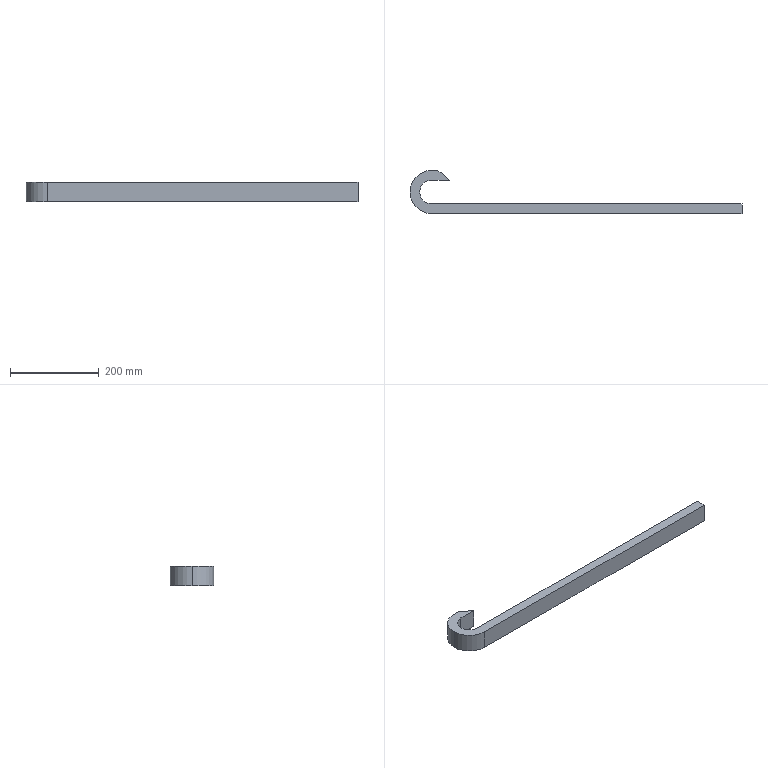Part | SolidWorks | features Cut 1, Extrusion 1 | 1 solid | 12 faces | box 749 x 98 x 43 mm | volume 800736 mm3 | plane 8 | cylinder 4 | commonest cylinder face diameters 54 x2 98 x2
STEP:
#1=CARTESIAN_POINT('',(-457.421,48.,43.));
#2=VERTEX_POINT('',#1);
#3=CARTESIAN_POINT('',(-408.421,-1.,43.));
#4=VERTEX_POINT('',#3);
#5=CARTESIAN_POINT('',(-408.421,48.,43.));
#6=DIRECTION('',(0.,0.,1.));
#7=DIRECTION('',(-1.,0.,0.));
#8=AXIS2_PLACEMENT_3D('',#5,#6,#7);
#9=CIRCLE('',#8,49.);
#10=EDGE_CURVE('',#2,#4,#9,.T.);
#11=ORIENTED_EDGE('',*,*,#10,.F.);
#12=CARTESIAN_POINT('',(-457.421,48.,0.));
#13=VERTEX_POINT('',#12);
#14=CARTESIAN_POINT('',(-457.421,48.,43.));
#15=DIRECTION('',(0.,0.,-1.));
#16=VECTOR('',#15,1000.);
#17=LINE('',#14,#16);
#18=EDGE_CURVE('',#2,#13,#17,.T.);
#19=ORIENTED_EDGE('',*,*,#18,.T.);
#20=CARTESIAN_POINT('',(-408.421,-1.,0.));
#21=VERTEX_POINT('',#20);
#22=CARTESIAN_POINT('',(-408.421,48.,0.));
#23=DIRECTION('',(0.,0.,1.));
#24=DIRECTION('',(-1.,0.,0.));
#25=AXIS2_PLACEMENT_3D('',#22,#23,#24);
#26=CIRCLE('',#25,49.);
#27=EDGE_CURVE('',#13,#21,#26,.T.);
#28=ORIENTED_EDGE('',*,*,#27,.T.);
#29=CARTESIAN_POINT('',(-408.421,-1.,43.));
#30=DIRECTION('',(0.,0.,-1.));
#31=VECTOR('',#30,1000.);
#32=LINE('',#29,#31);
#33=EDGE_CURVE('',#4,#21,#32,.T.);
#34=ORIENTED_EDGE('',*,*,#33,.F.);
#35=EDGE_LOOP('',(#11,#19,#28,#34));
#36=FACE_OUTER_BOUND('',#35,.T.);
#37=CARTESIAN_POINT('',(-408.421,48.,43.));
#38=DIRECTION('',(0.,0.,-1.));
#39=DIRECTION('',(-1.,0.,0.));
#40=AXIS2_PLACEMENT_3D('',#37,#38,#39);
#41=CYLINDRICAL_SURFACE('',#40,49.);
#42=ADVANCED_FACE('',(#36),#41,.T.);
#43=CARTESIAN_POINT('',(-435.421,48.,43.));
#44=VERTEX_POINT('',#43);
#45=CARTESIAN_POINT('',(-408.421,75.,43.));
#46=VERTEX_POINT('',#45);
#47=CARTESIAN_POINT('',(-408.421,48.,43.));
#48=DIRECTION('',(0.,0.,-1.));
#49=DIRECTION('',(1.,0.,0.));
#50=AXIS2_PLACEMENT_3D('',#47,#48,#49);
#51=CIRCLE('',#50,27.);
#52=EDGE_CURVE('',#44,#46,#51,.T.);
#53=ORIENTED_EDGE('',*,*,#52,.F.);
#54=CARTESIAN_POINT('',(-435.421,48.,0.));
#55=VERTEX_POINT('',#54);
#56=CARTESIAN_POINT('',(-435.421,48.,43.));
#57=DIRECTION('',(0.,0.,-1.));
#58=VECTOR('',#57,1000.);
#59=LINE('',#56,#58);
#60=EDGE_CURVE('',#44,#55,#59,.T.);
#61=ORIENTED_EDGE('',*,*,#60,.T.);
#62=CARTESIAN_POINT('',(-408.421,75.,0.));
#63=VERTEX_POINT('',#62);
#64=CARTESIAN_POINT('',(-408.421,48.,0.));
#65=DIRECTION('',(0.,0.,-1.));
#66=DIRECTION('',(1.,0.,0.));
#67=AXIS2_PLACEMENT_3D('',#64,#65,#66);
#68=CIRCLE('',#67,27.);
#69=EDGE_CURVE('',#55,#63,#68,.T.);
#70=ORIENTED_EDGE('',*,*,#69,.T.);
#71=CARTESIAN_POINT('',(-408.421,75.,43.));
#72=DIRECTION('',(0.,0.,-1.));
#73=VECTOR('',#72,1000.);
#74=LINE('',#71,#73);
#75=EDGE_CURVE('',#46,#63,#74,.T.);
#76=ORIENTED_EDGE('',*,*,#75,.F.);
#77=EDGE_LOOP('',(#53,#61,#70,#76));
#78=FACE_OUTER_BOUND('',#77,.T.);
#79=CARTESIAN_POINT('',(-408.421,48.,43.));
#80=DIRECTION('',(0.,0.,-1.));
#81=DIRECTION('',(-1.,0.,0.));
#82=AXIS2_PLACEMENT_3D('',#79,#80,#81);
#83=CYLINDRICAL_SURFACE('',#82,27.);
#84=ADVANCED_FACE('',(#78),#83,.F.);
#85=CARTESIAN_POINT('',(-368.343,75.,43.));
#86=VERTEX_POINT('',#85);
#87=CARTESIAN_POINT('',(-368.343,75.,0.));
#88=VERTEX_POINT('',#87);
#89=CARTESIAN_POINT('',(-368.343,75.,1042.509));
#90=DIRECTION('',(0.,0.,-1.));
#91=VECTOR('',#90,1000.);
#92=LINE('',#89,#91);
#93=EDGE_CURVE('',#86,#88,#92,.T.);
#94=ORIENTED_EDGE('',*,*,#93,.F.);
#95=CARTESIAN_POINT('',(-408.421,75.,43.));
#96=DIRECTION('',(1.,0.,0.));
#97=VECTOR('',#96,1000.);
#98=LINE('',#95,#97);
#99=EDGE_CURVE('',#46,#86,#98,.T.);
#100=ORIENTED_EDGE('',*,*,#99,.F.);
#101=ORIENTED_EDGE('',*,*,#75,.T.);
#102=CARTESIAN_POINT('',(-408.421,75.,0.));
#103=DIRECTION('',(1.,0.,0.));
#104=VECTOR('',#103,1000.);
#105=LINE('',#102,#104);
#106=EDGE_CURVE('',#63,#88,#105,.T.);
#107=ORIENTED_EDGE('',*,*,#106,.T.);
#108=EDGE_LOOP('',(#94,#100,#101,#107));
#109=FACE_OUTER_BOUND('',#108,.T.);
#110=CARTESIAN_POINT('',(-408.421,75.,43.));
#111=DIRECTION('',(0.,1.,0.));
#112=DIRECTION('',(0.,0.,1.));
#113=AXIS2_PLACEMENT_3D('',#110,#111,#112);
#114=PLANE('',#113);
#115=ADVANCED_FACE('',(#109),#114,.F.);
#116=CARTESIAN_POINT('',(-394.373,97.,43.));
#117=VERTEX_POINT('',#116);
#118=CARTESIAN_POINT('',(-394.373,97.,0.));
#119=VERTEX_POINT('',#118);
#120=CARTESIAN_POINT('',(-394.373,97.,1042.509));
#121=DIRECTION('',(0.,0.,-1.));
#122=VECTOR('',#121,1000.);
#123=LINE('',#120,#122);
#124=EDGE_CURVE('',#117,#119,#123,.T.);
#125=ORIENTED_EDGE('',*,*,#124,.T.);
#126=CARTESIAN_POINT('',(-408.421,97.,0.));
#127=VERTEX_POINT('',#126);
#128=CARTESIAN_POINT('',(-408.421,97.,0.));
#129=DIRECTION('',(-1.,0.,0.));
#130=VECTOR('',#129,1000.);
#131=LINE('',#128,#130);
#132=EDGE_CURVE('',#119,#127,#131,.T.);
#133=ORIENTED_EDGE('',*,*,#132,.T.);
#134=CARTESIAN_POINT('',(-408.421,97.,43.));
#135=VERTEX_POINT('',#134);
#136=CARTESIAN_POINT('',(-408.421,97.,43.));
#137=DIRECTION('',(0.,0.,-1.));
#138=VECTOR('',#137,1000.);
#139=LINE('',#136,#138);
#140=EDGE_CURVE('',#135,#127,#139,.T.);
#141=ORIENTED_EDGE('',*,*,#140,.F.);
#142=CARTESIAN_POINT('',(-408.421,97.,43.));
#143=DIRECTION('',(-1.,0.,0.));
#144=VECTOR('',#143,1000.);
#145=LINE('',#142,#144);
#146=EDGE_CURVE('',#117,#135,#145,.T.);
#147=ORIENTED_EDGE('',*,*,#146,.F.);
#148=EDGE_LOOP('',(#125,#133,#141,#147));
#149=FACE_OUTER_BOUND('',#148,.T.);
#150=CARTESIAN_POINT('',(-408.421,97.,43.));
#151=DIRECTION('',(0.,-1.,0.));
#152=DIRECTION('',(1.,0.,0.));
#153=AXIS2_PLACEMENT_3D('',#150,#151,#152);
#154=PLANE('',#153);
#155=ADVANCED_FACE('',(#149),#154,.F.);
#156=ORIENTED_EDGE('',*,*,#99,.T.);
#157=CARTESIAN_POINT('',(-378.411,83.509,43.));
#158=DIRECTION('',(-0.7638,0.6455,0.));
#159=VECTOR('',#158,1000.);
#160=LINE('',#157,#159);
#161=EDGE_CURVE('',#86,#117,#160,.T.);
#162=ORIENTED_EDGE('',*,*,#161,.T.);
#163=ORIENTED_EDGE('',*,*,#146,.T.);
#164=CARTESIAN_POINT('',(-408.421,48.,43.));
#165=DIRECTION('',(0.,0.,1.));
#166=DIRECTION('',(-1.,0.,0.));
#167=AXIS2_PLACEMENT_3D('',#164,#165,#166);
#168=CIRCLE('',#167,49.);
#169=EDGE_CURVE('',#135,#2,#168,.T.);
#170=ORIENTED_EDGE('',*,*,#169,.T.);
#171=ORIENTED_EDGE('',*,*,#10,.T.);
#172=CARTESIAN_POINT('',(291.579,-1.,43.));
#173=VERTEX_POINT('',#172);
#174=CARTESIAN_POINT('',(291.579,-1.,43.));
#175=DIRECTION('',(1.,0.,0.));
#176=VECTOR('',#175,1000.);
#177=LINE('',#174,#176);
#178=EDGE_CURVE('',#4,#173,#177,.T.);
#179=ORIENTED_EDGE('',*,*,#178,.T.);
#180=CARTESIAN_POINT('',(291.579,21.,43.));
#181=VERTEX_POINT('',#180);
#182=CARTESIAN_POINT('',(291.579,-1.,43.));
#183=DIRECTION('',(0.,1.,0.));
#184=VECTOR('',#183,1000.);
#185=LINE('',#182,#184);
#186=EDGE_CURVE('',#173,#181,#185,.T.);
#187=ORIENTED_EDGE('',*,*,#186,.T.);
#188=CARTESIAN_POINT('',(-408.421,21.,43.));
#189=VERTEX_POINT('',#188);
#190=CARTESIAN_POINT('',(291.579,21.,43.));
#191=DIRECTION('',(-1.,0.,0.));
#192=VECTOR('',#191,1000.);
#193=LINE('',#190,#192);
#194=EDGE_CURVE('',#181,#189,#193,.T.);
#195=ORIENTED_EDGE('',*,*,#194,.T.);
#196=CARTESIAN_POINT('',(-408.421,48.,43.));
#197=DIRECTION('',(0.,0.,-1.));
#198=DIRECTION('',(1.,0.,0.));
#199=AXIS2_PLACEMENT_3D('',#196,#197,#198);
#200=CIRCLE('',#199,27.);
#201=EDGE_CURVE('',#189,#44,#200,.T.);
#202=ORIENTED_EDGE('',*,*,#201,.T.);
#203=ORIENTED_EDGE('',*,*,#52,.T.);
#204=EDGE_LOOP('',(#156,#162,#163,#170,#171,#179,#187,#195,#202,#203));
#205=FACE_OUTER_BOUND('',#204,.T.);
#206=CARTESIAN_POINT('',(-408.421,48.,43.));
#207=DIRECTION('',(0.,0.,1.));
#208=DIRECTION('',(1.,0.,0.));
#209=AXIS2_PLACEMENT_3D('',#206,#207,#208);
#210=PLANE('',#209);
#211=ADVANCED_FACE('',(#205),#210,.T.);
#212=CARTESIAN_POINT('',(-378.411,83.509,0.));
#213=DIRECTION('',(-0.7638,0.6455,0.));
#214=VECTOR('',#213,1000.);
#215=LINE('',#212,#214);
#216=EDGE_CURVE('',#88,#119,#215,.T.);
#217=ORIENTED_EDGE('',*,*,#216,.F.);
#218=ORIENTED_EDGE('',*,*,#106,.F.);
#219=ORIENTED_EDGE('',*,*,#69,.F.);
#220=CARTESIAN_POINT('',(-408.421,21.,0.));
#221=VERTEX_POINT('',#220);
#222=CARTESIAN_POINT('',(-408.421,48.,0.));
#223=DIRECTION('',(0.,0.,-1.));
#224=DIRECTION('',(1.,0.,0.));
#225=AXIS2_PLACEMENT_3D('',#222,#223,#224);
#226=CIRCLE('',#225,27.);
#227=EDGE_CURVE('',#221,#55,#226,.T.);
#228=ORIENTED_EDGE('',*,*,#227,.F.);
#229=CARTESIAN_POINT('',(291.579,21.,0.));
#230=VERTEX_POINT('',#229);
#231=CARTESIAN_POINT('',(291.579,21.,0.));
#232=DIRECTION('',(-1.,0.,0.));
#233=VECTOR('',#232,1000.);
#234=LINE('',#231,#233);
#235=EDGE_CURVE('',#230,#221,#234,.T.);
#236=ORIENTED_EDGE('',*,*,#235,.F.);
#237=CARTESIAN_POINT('',(291.579,-1.,0.));
#238=VERTEX_POINT('',#237);
#239=CARTESIAN_POINT('',(291.579,-1.,0.));
#240=DIRECTION('',(0.,1.,0.));
#241=VECTOR('',#240,1000.);
#242=LINE('',#239,#241);
#243=EDGE_CURVE('',#238,#230,#242,.T.);
#244=ORIENTED_EDGE('',*,*,#243,.F.);
#245=CARTESIAN_POINT('',(291.579,-1.,0.));
#246=DIRECTION('',(1.,0.,0.));
#247=VECTOR('',#246,1000.);
#248=LINE('',#245,#247);
#249=EDGE_CURVE('',#21,#238,#248,.T.);
#250=ORIENTED_EDGE('',*,*,#249,.F.);
#251=ORIENTED_EDGE('',*,*,#27,.F.);
#252=CARTESIAN_POINT('',(-408.421,48.,0.));
#253=DIRECTION('',(0.,0.,1.));
#254=DIRECTION('',(-1.,0.,0.));
#255=AXIS2_PLACEMENT_3D('',#252,#253,#254);
#256=CIRCLE('',#255,49.);
#257=EDGE_CURVE('',#127,#13,#256,.T.);
#258=ORIENTED_EDGE('',*,*,#257,.F.);
#259=ORIENTED_EDGE('',*,*,#132,.F.);
#260=EDGE_LOOP('',(#217,#218,#219,#228,#236,#244,#250,#251,#258,#259));
#261=FACE_OUTER_BOUND('',#260,.T.);
#262=CARTESIAN_POINT('',(-408.421,48.,0.));
#263=DIRECTION('',(0.,0.,1.));
#264=DIRECTION('',(1.,0.,0.));
#265=AXIS2_PLACEMENT_3D('',#262,#263,#264);
#266=PLANE('',#265);
#267=ADVANCED_FACE('',(#261),#266,.F.);
#268=ORIENTED_EDGE('',*,*,#243,.T.);
#269=CARTESIAN_POINT('',(291.579,21.,43.));
#270=DIRECTION('',(0.,0.,-1.));
#271=VECTOR('',#270,1000.);
#272=LINE('',#269,#271);
#273=EDGE_CURVE('',#181,#230,#272,.T.);
#274=ORIENTED_EDGE('',*,*,#273,.F.);
#275=ORIENTED_EDGE('',*,*,#186,.F.);
#276=CARTESIAN_POINT('',(291.579,-1.,43.));
#277=DIRECTION('',(0.,0.,-1.));
#278=VECTOR('',#277,1000.);
#279=LINE('',#276,#278);
#280=EDGE_CURVE('',#173,#238,#279,.T.);
#281=ORIENTED_EDGE('',*,*,#280,.T.);
#282=EDGE_LOOP('',(#268,#274,#275,#281));
#283=FACE_OUTER_BOUND('',#282,.T.);
#284=CARTESIAN_POINT('',(291.579,-1.,43.));
#285=DIRECTION('',(-1.,0.,0.));
#286=DIRECTION('',(0.,-1.,0.));
#287=AXIS2_PLACEMENT_3D('',#284,#285,#286);
#288=PLANE('',#287);
#289=ADVANCED_FACE('',(#283),#288,.F.);
#290=ORIENTED_EDGE('',*,*,#235,.T.);
#291=CARTESIAN_POINT('',(-408.421,21.,43.));
#292=DIRECTION('',(0.,0.,-1.));
#293=VECTOR('',#292,1000.);
#294=LINE('',#291,#293);
#295=EDGE_CURVE('',#189,#221,#294,.T.);
#296=ORIENTED_EDGE('',*,*,#295,.F.);
#297=ORIENTED_EDGE('',*,*,#194,.F.);
#298=ORIENTED_EDGE('',*,*,#273,.T.);
#299=EDGE_LOOP('',(#290,#296,#297,#298));
#300=FACE_OUTER_BOUND('',#299,.T.);
#301=CARTESIAN_POINT('',(291.579,21.,43.));
#302=DIRECTION('',(0.,-1.,0.));
#303=DIRECTION('',(1.,0.,0.));
#304=AXIS2_PLACEMENT_3D('',#301,#302,#303);
#305=PLANE('',#304);
#306=ADVANCED_FACE('',(#300),#305,.F.);
#307=ORIENTED_EDGE('',*,*,#60,.F.);
#308=ORIENTED_EDGE('',*,*,#201,.F.);
#309=ORIENTED_EDGE('',*,*,#295,.T.);
#310=ORIENTED_EDGE('',*,*,#227,.T.);
#311=EDGE_LOOP('',(#307,#308,#309,#310));
#312=FACE_OUTER_BOUND('',#311,.T.);
#313=CARTESIAN_POINT('',(-408.421,48.,43.));
#314=DIRECTION('',(0.,0.,-1.));
#315=DIRECTION('',(-1.,0.,0.));
#316=AXIS2_PLACEMENT_3D('',#313,#314,#315);
#317=CYLINDRICAL_SURFACE('',#316,27.);
#318=ADVANCED_FACE('',(#312),#317,.F.);
#319=ORIENTED_EDGE('',*,*,#18,.F.);
#320=ORIENTED_EDGE('',*,*,#169,.F.);
#321=ORIENTED_EDGE('',*,*,#140,.T.);
#322=ORIENTED_EDGE('',*,*,#257,.T.);
#323=EDGE_LOOP('',(#319,#320,#321,#322));
#324=FACE_OUTER_BOUND('',#323,.T.);
#325=CARTESIAN_POINT('',(-408.421,48.,43.));
#326=DIRECTION('',(0.,0.,-1.));
#327=DIRECTION('',(-1.,0.,0.));
#328=AXIS2_PLACEMENT_3D('',#325,#326,#327);
#329=CYLINDRICAL_SURFACE('',#328,49.);
#330=ADVANCED_FACE('',(#324),#329,.T.);
#331=ORIENTED_EDGE('',*,*,#249,.T.);
#332=ORIENTED_EDGE('',*,*,#280,.F.);
#333=ORIENTED_EDGE('',*,*,#178,.F.);
#334=ORIENTED_EDGE('',*,*,#33,.T.);
#335=EDGE_LOOP('',(#331,#332,#333,#334));
#336=FACE_OUTER_BOUND('',#335,.T.);
#337=CARTESIAN_POINT('',(291.579,-1.,43.));
#338=DIRECTION('',(0.,1.,0.));
#339=DIRECTION('',(-1.,0.,0.));
#340=AXIS2_PLACEMENT_3D('',#337,#338,#339);
#341=PLANE('',#340);
#342=ADVANCED_FACE('',(#336),#341,.F.);
#343=ORIENTED_EDGE('',*,*,#161,.F.);
#344=ORIENTED_EDGE('',*,*,#93,.T.);
#345=ORIENTED_EDGE('',*,*,#216,.T.);
#346=ORIENTED_EDGE('',*,*,#124,.F.);
#347=EDGE_LOOP('',(#343,#344,#345,#346));
#348=FACE_OUTER_BOUND('',#347,.T.);
#349=CARTESIAN_POINT('',(-394.373,97.,1042.509));
#350=DIRECTION('',(0.6455,0.7638,0.));
#351=DIRECTION('',(-0.7638,0.6455,0.));
#352=AXIS2_PLACEMENT_3D('',#349,#350,#351);
#353=PLANE('',#352);
#354=ADVANCED_FACE('',(#348),#353,.T.);
#355=CLOSED_SHELL('',(#42,#84,#115,#155,#211,#267,#289,#306,#318,#330,#342,#354));
#356=MANIFOLD_SOLID_BREP('',#355);
#357=CARTESIAN_POINT('',(0.,0.,0.));
#358=DIRECTION('',(0.,0.,1.));
#359=DIRECTION('',(1.,0.,0.));
#360=AXIS2_PLACEMENT_3D('',#357,#358,#359);
#361=(LENGTH_UNIT()NAMED_UNIT(*)SI_UNIT(.MILLI.,.METRE.));
#362=UNCERTAINTY_MEASURE_WITH_UNIT(LENGTH_MEASURE(0.00001),#361,'','');
#363=(NAMED_UNIT(*)PLANE_ANGLE_UNIT()SI_UNIT($,.RADIAN.));
#364=(NAMED_UNIT(*)SI_UNIT($,.STERADIAN.)SOLID_ANGLE_UNIT());
#365=(GEOMETRIC_REPRESENTATION_CONTEXT(3)GLOBAL_UNCERTAINTY_ASSIGNED_CONTEXT((#362))GLOBAL_UNIT_ASSIGNED_CONTEXT((#361,#363,#364))REPRESENTATION_CONTEXT('',''));
#366=ADVANCED_BREP_SHAPE_REPRESENTATION('',(#356,#360),#365);